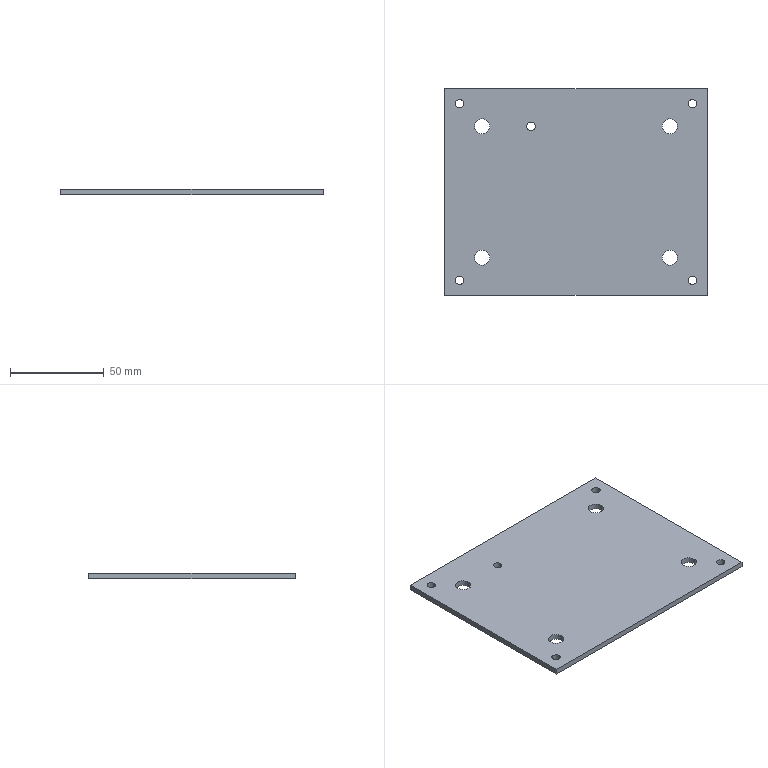Part | SolidWorks | features Extrusion 1 | 1 solid | 24 faces | box 140 x 110 x 3 mm | volume 45343 mm3 | cylinder 18 | plane 6 | commonest cylinder face diameters 4.5 x10 8.1 x8
STEP:
#1=CARTESIAN_POINT('',(-26.25,35.,-1.5));
#2=VERTEX_POINT('',#1);
#3=CARTESIAN_POINT('',(-21.75,35.,-1.5));
#4=VERTEX_POINT('',#3);
#5=CARTESIAN_POINT('',(-24.,35.,-1.5));
#6=DIRECTION('',(0.,0.,1.));
#7=DIRECTION('',(1.,0.,0.));
#8=AXIS2_PLACEMENT_3D('',#5,#6,#7);
#9=CIRCLE('',#8,2.25);
#10=EDGE_CURVE('',#2,#4,#9,.T.);
#11=ORIENTED_EDGE('',*,*,#10,.F.);
#12=CARTESIAN_POINT('',(-26.25,35.,1.5));
#13=VERTEX_POINT('',#12);
#14=CARTESIAN_POINT('',(-26.25,35.,-1.5));
#15=DIRECTION('',(0.,0.,1.));
#16=VECTOR('',#15,1000.);
#17=LINE('',#14,#16);
#18=EDGE_CURVE('',#2,#13,#17,.T.);
#19=ORIENTED_EDGE('',*,*,#18,.T.);
#20=CARTESIAN_POINT('',(-21.75,35.,1.5));
#21=VERTEX_POINT('',#20);
#22=CARTESIAN_POINT('',(-24.,35.,1.5));
#23=DIRECTION('',(0.,0.,1.));
#24=DIRECTION('',(1.,0.,0.));
#25=AXIS2_PLACEMENT_3D('',#22,#23,#24);
#26=CIRCLE('',#25,2.25);
#27=EDGE_CURVE('',#13,#21,#26,.T.);
#28=ORIENTED_EDGE('',*,*,#27,.T.);
#29=CARTESIAN_POINT('',(-21.75,35.,-1.5));
#30=DIRECTION('',(0.,0.,1.));
#31=VECTOR('',#30,1000.);
#32=LINE('',#29,#31);
#33=EDGE_CURVE('',#4,#21,#32,.T.);
#34=ORIENTED_EDGE('',*,*,#33,.F.);
#35=EDGE_LOOP('',(#11,#19,#28,#34));
#36=FACE_OUTER_BOUND('',#35,.T.);
#37=CARTESIAN_POINT('',(-24.,35.,-1.5));
#38=DIRECTION('',(0.,0.,1.));
#39=DIRECTION('',(1.,0.,0.));
#40=AXIS2_PLACEMENT_3D('',#37,#38,#39);
#41=CYLINDRICAL_SURFACE('',#40,2.25);
#42=ADVANCED_FACE('',(#36),#41,.F.);
#43=CARTESIAN_POINT('',(45.95,35.,-1.5));
#44=VERTEX_POINT('',#43);
#45=CARTESIAN_POINT('',(54.05,35.,-1.5));
#46=VERTEX_POINT('',#45);
#47=CARTESIAN_POINT('',(50.,35.,-1.5));
#48=DIRECTION('',(0.,0.,1.));
#49=DIRECTION('',(1.,0.,0.));
#50=AXIS2_PLACEMENT_3D('',#47,#48,#49);
#51=CIRCLE('',#50,4.05);
#52=EDGE_CURVE('',#44,#46,#51,.T.);
#53=ORIENTED_EDGE('',*,*,#52,.F.);
#54=CARTESIAN_POINT('',(45.95,35.,1.5));
#55=VERTEX_POINT('',#54);
#56=CARTESIAN_POINT('',(45.95,35.,-1.5));
#57=DIRECTION('',(0.,0.,1.));
#58=VECTOR('',#57,1000.);
#59=LINE('',#56,#58);
#60=EDGE_CURVE('',#44,#55,#59,.T.);
#61=ORIENTED_EDGE('',*,*,#60,.T.);
#62=CARTESIAN_POINT('',(54.05,35.,1.5));
#63=VERTEX_POINT('',#62);
#64=CARTESIAN_POINT('',(50.,35.,1.5));
#65=DIRECTION('',(0.,0.,1.));
#66=DIRECTION('',(1.,0.,0.));
#67=AXIS2_PLACEMENT_3D('',#64,#65,#66);
#68=CIRCLE('',#67,4.05);
#69=EDGE_CURVE('',#55,#63,#68,.T.);
#70=ORIENTED_EDGE('',*,*,#69,.T.);
#71=CARTESIAN_POINT('',(54.05,35.,-1.5));
#72=DIRECTION('',(0.,0.,1.));
#73=VECTOR('',#72,1000.);
#74=LINE('',#71,#73);
#75=EDGE_CURVE('',#46,#63,#74,.T.);
#76=ORIENTED_EDGE('',*,*,#75,.F.);
#77=EDGE_LOOP('',(#53,#61,#70,#76));
#78=FACE_OUTER_BOUND('',#77,.T.);
#79=CARTESIAN_POINT('',(50.,35.,-1.5));
#80=DIRECTION('',(0.,0.,1.));
#81=DIRECTION('',(1.,0.,0.));
#82=AXIS2_PLACEMENT_3D('',#79,#80,#81);
#83=CYLINDRICAL_SURFACE('',#82,4.05);
#84=ADVANCED_FACE('',(#78),#83,.F.);
#85=CARTESIAN_POINT('',(45.95,-35.,-1.5));
#86=VERTEX_POINT('',#85);
#87=CARTESIAN_POINT('',(54.05,-35.,-1.5));
#88=VERTEX_POINT('',#87);
#89=CARTESIAN_POINT('',(50.,-35.,-1.5));
#90=DIRECTION('',(0.,0.,1.));
#91=DIRECTION('',(1.,0.,0.));
#92=AXIS2_PLACEMENT_3D('',#89,#90,#91);
#93=CIRCLE('',#92,4.05);
#94=EDGE_CURVE('',#86,#88,#93,.T.);
#95=ORIENTED_EDGE('',*,*,#94,.F.);
#96=CARTESIAN_POINT('',(45.95,-35.,1.5));
#97=VERTEX_POINT('',#96);
#98=CARTESIAN_POINT('',(45.95,-35.,-1.5));
#99=DIRECTION('',(0.,0.,1.));
#100=VECTOR('',#99,1000.);
#101=LINE('',#98,#100);
#102=EDGE_CURVE('',#86,#97,#101,.T.);
#103=ORIENTED_EDGE('',*,*,#102,.T.);
#104=CARTESIAN_POINT('',(54.05,-35.,1.5));
#105=VERTEX_POINT('',#104);
#106=CARTESIAN_POINT('',(50.,-35.,1.5));
#107=DIRECTION('',(0.,0.,1.));
#108=DIRECTION('',(1.,0.,0.));
#109=AXIS2_PLACEMENT_3D('',#106,#107,#108);
#110=CIRCLE('',#109,4.05);
#111=EDGE_CURVE('',#97,#105,#110,.T.);
#112=ORIENTED_EDGE('',*,*,#111,.T.);
#113=CARTESIAN_POINT('',(54.05,-35.,-1.5));
#114=DIRECTION('',(0.,0.,1.));
#115=VECTOR('',#114,1000.);
#116=LINE('',#113,#115);
#117=EDGE_CURVE('',#88,#105,#116,.T.);
#118=ORIENTED_EDGE('',*,*,#117,.F.);
#119=EDGE_LOOP('',(#95,#103,#112,#118));
#120=FACE_OUTER_BOUND('',#119,.T.);
#121=CARTESIAN_POINT('',(50.,-35.,-1.5));
#122=DIRECTION('',(0.,0.,1.));
#123=DIRECTION('',(1.,0.,0.));
#124=AXIS2_PLACEMENT_3D('',#121,#122,#123);
#125=CYLINDRICAL_SURFACE('',#124,4.05);
#126=ADVANCED_FACE('',(#120),#125,.F.);
#127=CARTESIAN_POINT('',(-54.05,35.,-1.5));
#128=VERTEX_POINT('',#127);
#129=CARTESIAN_POINT('',(-45.95,35.,-1.5));
#130=VERTEX_POINT('',#129);
#131=CARTESIAN_POINT('',(-50.,35.,-1.5));
#132=DIRECTION('',(0.,0.,1.));
#133=DIRECTION('',(1.,0.,0.));
#134=AXIS2_PLACEMENT_3D('',#131,#132,#133);
#135=CIRCLE('',#134,4.05);
#136=EDGE_CURVE('',#128,#130,#135,.T.);
#137=ORIENTED_EDGE('',*,*,#136,.F.);
#138=CARTESIAN_POINT('',(-54.05,35.,1.5));
#139=VERTEX_POINT('',#138);
#140=CARTESIAN_POINT('',(-54.05,35.,-1.5));
#141=DIRECTION('',(0.,0.,1.));
#142=VECTOR('',#141,1000.);
#143=LINE('',#140,#142);
#144=EDGE_CURVE('',#128,#139,#143,.T.);
#145=ORIENTED_EDGE('',*,*,#144,.T.);
#146=CARTESIAN_POINT('',(-45.95,35.,1.5));
#147=VERTEX_POINT('',#146);
#148=CARTESIAN_POINT('',(-50.,35.,1.5));
#149=DIRECTION('',(0.,0.,1.));
#150=DIRECTION('',(1.,0.,0.));
#151=AXIS2_PLACEMENT_3D('',#148,#149,#150);
#152=CIRCLE('',#151,4.05);
#153=EDGE_CURVE('',#139,#147,#152,.T.);
#154=ORIENTED_EDGE('',*,*,#153,.T.);
#155=CARTESIAN_POINT('',(-45.95,35.,-1.5));
#156=DIRECTION('',(0.,0.,1.));
#157=VECTOR('',#156,1000.);
#158=LINE('',#155,#157);
#159=EDGE_CURVE('',#130,#147,#158,.T.);
#160=ORIENTED_EDGE('',*,*,#159,.F.);
#161=EDGE_LOOP('',(#137,#145,#154,#160));
#162=FACE_OUTER_BOUND('',#161,.T.);
#163=CARTESIAN_POINT('',(-50.,35.,-1.5));
#164=DIRECTION('',(0.,0.,1.));
#165=DIRECTION('',(1.,0.,0.));
#166=AXIS2_PLACEMENT_3D('',#163,#164,#165);
#167=CYLINDRICAL_SURFACE('',#166,4.05);
#168=ADVANCED_FACE('',(#162),#167,.F.);
#169=CARTESIAN_POINT('',(-54.05,-35.,-1.5));
#170=VERTEX_POINT('',#169);
#171=CARTESIAN_POINT('',(-45.95,-35.,-1.5));
#172=VERTEX_POINT('',#171);
#173=CARTESIAN_POINT('',(-50.,-35.,-1.5));
#174=DIRECTION('',(0.,0.,1.));
#175=DIRECTION('',(1.,0.,0.));
#176=AXIS2_PLACEMENT_3D('',#173,#174,#175);
#177=CIRCLE('',#176,4.05);
#178=EDGE_CURVE('',#170,#172,#177,.T.);
#179=ORIENTED_EDGE('',*,*,#178,.F.);
#180=CARTESIAN_POINT('',(-54.05,-35.,1.5));
#181=VERTEX_POINT('',#180);
#182=CARTESIAN_POINT('',(-54.05,-35.,-1.5));
#183=DIRECTION('',(0.,0.,1.));
#184=VECTOR('',#183,1000.);
#185=LINE('',#182,#184);
#186=EDGE_CURVE('',#170,#181,#185,.T.);
#187=ORIENTED_EDGE('',*,*,#186,.T.);
#188=CARTESIAN_POINT('',(-45.95,-35.,1.5));
#189=VERTEX_POINT('',#188);
#190=CARTESIAN_POINT('',(-50.,-35.,1.5));
#191=DIRECTION('',(0.,0.,1.));
#192=DIRECTION('',(1.,0.,0.));
#193=AXIS2_PLACEMENT_3D('',#190,#191,#192);
#194=CIRCLE('',#193,4.05);
#195=EDGE_CURVE('',#181,#189,#194,.T.);
#196=ORIENTED_EDGE('',*,*,#195,.T.);
#197=CARTESIAN_POINT('',(-45.95,-35.,-1.5));
#198=DIRECTION('',(0.,0.,1.));
#199=VECTOR('',#198,1000.);
#200=LINE('',#197,#199);
#201=EDGE_CURVE('',#172,#189,#200,.T.);
#202=ORIENTED_EDGE('',*,*,#201,.F.);
#203=EDGE_LOOP('',(#179,#187,#196,#202));
#204=FACE_OUTER_BOUND('',#203,.T.);
#205=CARTESIAN_POINT('',(-50.,-35.,-1.5));
#206=DIRECTION('',(0.,0.,1.));
#207=DIRECTION('',(1.,0.,0.));
#208=AXIS2_PLACEMENT_3D('',#205,#206,#207);
#209=CYLINDRICAL_SURFACE('',#208,4.05);
#210=ADVANCED_FACE('',(#204),#209,.F.);
#211=CARTESIAN_POINT('',(59.75,47.,-1.5));
#212=VERTEX_POINT('',#211);
#213=CARTESIAN_POINT('',(64.25,47.,-1.5));
#214=VERTEX_POINT('',#213);
#215=CARTESIAN_POINT('',(62.,47.,-1.5));
#216=DIRECTION('',(0.,0.,1.));
#217=DIRECTION('',(1.,0.,0.));
#218=AXIS2_PLACEMENT_3D('',#215,#216,#217);
#219=CIRCLE('',#218,2.25);
#220=EDGE_CURVE('',#212,#214,#219,.T.);
#221=ORIENTED_EDGE('',*,*,#220,.F.);
#222=CARTESIAN_POINT('',(59.75,47.,1.5));
#223=VERTEX_POINT('',#222);
#224=CARTESIAN_POINT('',(59.75,47.,-1.5));
#225=DIRECTION('',(0.,0.,1.));
#226=VECTOR('',#225,1000.);
#227=LINE('',#224,#226);
#228=EDGE_CURVE('',#212,#223,#227,.T.);
#229=ORIENTED_EDGE('',*,*,#228,.T.);
#230=CARTESIAN_POINT('',(64.25,47.,1.5));
#231=VERTEX_POINT('',#230);
#232=CARTESIAN_POINT('',(62.,47.,1.5));
#233=DIRECTION('',(0.,0.,1.));
#234=DIRECTION('',(1.,0.,0.));
#235=AXIS2_PLACEMENT_3D('',#232,#233,#234);
#236=CIRCLE('',#235,2.25);
#237=EDGE_CURVE('',#223,#231,#236,.T.);
#238=ORIENTED_EDGE('',*,*,#237,.T.);
#239=CARTESIAN_POINT('',(64.25,47.,-1.5));
#240=DIRECTION('',(0.,0.,1.));
#241=VECTOR('',#240,1000.);
#242=LINE('',#239,#241);
#243=EDGE_CURVE('',#214,#231,#242,.T.);
#244=ORIENTED_EDGE('',*,*,#243,.F.);
#245=EDGE_LOOP('',(#221,#229,#238,#244));
#246=FACE_OUTER_BOUND('',#245,.T.);
#247=CARTESIAN_POINT('',(62.,47.,-1.5));
#248=DIRECTION('',(0.,0.,1.));
#249=DIRECTION('',(1.,0.,0.));
#250=AXIS2_PLACEMENT_3D('',#247,#248,#249);
#251=CYLINDRICAL_SURFACE('',#250,2.25);
#252=ADVANCED_FACE('',(#246),#251,.F.);
#253=CARTESIAN_POINT('',(59.75,-47.,-1.5));
#254=VERTEX_POINT('',#253);
#255=CARTESIAN_POINT('',(64.25,-47.,-1.5));
#256=VERTEX_POINT('',#255);
#257=CARTESIAN_POINT('',(62.,-47.,-1.5));
#258=DIRECTION('',(0.,0.,1.));
#259=DIRECTION('',(1.,0.,0.));
#260=AXIS2_PLACEMENT_3D('',#257,#258,#259);
#261=CIRCLE('',#260,2.25);
#262=EDGE_CURVE('',#254,#256,#261,.T.);
#263=ORIENTED_EDGE('',*,*,#262,.F.);
#264=CARTESIAN_POINT('',(59.75,-47.,1.5));
#265=VERTEX_POINT('',#264);
#266=CARTESIAN_POINT('',(59.75,-47.,-1.5));
#267=DIRECTION('',(0.,0.,1.));
#268=VECTOR('',#267,1000.);
#269=LINE('',#266,#268);
#270=EDGE_CURVE('',#254,#265,#269,.T.);
#271=ORIENTED_EDGE('',*,*,#270,.T.);
#272=CARTESIAN_POINT('',(64.25,-47.,1.5));
#273=VERTEX_POINT('',#272);
#274=CARTESIAN_POINT('',(62.,-47.,1.5));
#275=DIRECTION('',(0.,0.,1.));
#276=DIRECTION('',(1.,0.,0.));
#277=AXIS2_PLACEMENT_3D('',#274,#275,#276);
#278=CIRCLE('',#277,2.25);
#279=EDGE_CURVE('',#265,#273,#278,.T.);
#280=ORIENTED_EDGE('',*,*,#279,.T.);
#281=CARTESIAN_POINT('',(64.25,-47.,-1.5));
#282=DIRECTION('',(0.,0.,1.));
#283=VECTOR('',#282,1000.);
#284=LINE('',#281,#283);
#285=EDGE_CURVE('',#256,#273,#284,.T.);
#286=ORIENTED_EDGE('',*,*,#285,.F.);
#287=EDGE_LOOP('',(#263,#271,#280,#286));
#288=FACE_OUTER_BOUND('',#287,.T.);
#289=CARTESIAN_POINT('',(62.,-47.,-1.5));
#290=DIRECTION('',(0.,0.,1.));
#291=DIRECTION('',(1.,0.,0.));
#292=AXIS2_PLACEMENT_3D('',#289,#290,#291);
#293=CYLINDRICAL_SURFACE('',#292,2.25);
#294=ADVANCED_FACE('',(#288),#293,.F.);
#295=CARTESIAN_POINT('',(-64.25,47.,-1.5));
#296=VERTEX_POINT('',#295);
#297=CARTESIAN_POINT('',(-59.75,47.,-1.5));
#298=VERTEX_POINT('',#297);
#299=CARTESIAN_POINT('',(-62.,47.,-1.5));
#300=DIRECTION('',(0.,0.,1.));
#301=DIRECTION('',(1.,0.,0.));
#302=AXIS2_PLACEMENT_3D('',#299,#300,#301);
#303=CIRCLE('',#302,2.25);
#304=EDGE_CURVE('',#296,#298,#303,.T.);
#305=ORIENTED_EDGE('',*,*,#304,.F.);
#306=CARTESIAN_POINT('',(-64.25,47.,1.5));
#307=VERTEX_POINT('',#306);
#308=CARTESIAN_POINT('',(-64.25,47.,-1.5));
#309=DIRECTION('',(0.,0.,1.));
#310=VECTOR('',#309,1000.);
#311=LINE('',#308,#310);
#312=EDGE_CURVE('',#296,#307,#311,.T.);
#313=ORIENTED_EDGE('',*,*,#312,.T.);
#314=CARTESIAN_POINT('',(-59.75,47.,1.5));
#315=VERTEX_POINT('',#314);
#316=CARTESIAN_POINT('',(-62.,47.,1.5));
#317=DIRECTION('',(0.,0.,1.));
#318=DIRECTION('',(1.,0.,0.));
#319=AXIS2_PLACEMENT_3D('',#316,#317,#318);
#320=CIRCLE('',#319,2.25);
#321=EDGE_CURVE('',#307,#315,#320,.T.);
#322=ORIENTED_EDGE('',*,*,#321,.T.);
#323=CARTESIAN_POINT('',(-59.75,47.,-1.5));
#324=DIRECTION('',(0.,0.,1.));
#325=VECTOR('',#324,1000.);
#326=LINE('',#323,#325);
#327=EDGE_CURVE('',#298,#315,#326,.T.);
#328=ORIENTED_EDGE('',*,*,#327,.F.);
#329=EDGE_LOOP('',(#305,#313,#322,#328));
#330=FACE_OUTER_BOUND('',#329,.T.);
#331=CARTESIAN_POINT('',(-62.,47.,-1.5));
#332=DIRECTION('',(0.,0.,1.));
#333=DIRECTION('',(1.,0.,0.));
#334=AXIS2_PLACEMENT_3D('',#331,#332,#333);
#335=CYLINDRICAL_SURFACE('',#334,2.25);
#336=ADVANCED_FACE('',(#330),#335,.F.);
#337=CARTESIAN_POINT('',(-64.25,-47.,-1.5));
#338=VERTEX_POINT('',#337);
#339=CARTESIAN_POINT('',(-59.75,-47.,-1.5));
#340=VERTEX_POINT('',#339);
#341=CARTESIAN_POINT('',(-62.,-47.,-1.5));
#342=DIRECTION('',(0.,0.,1.));
#343=DIRECTION('',(1.,0.,0.));
#344=AXIS2_PLACEMENT_3D('',#341,#342,#343);
#345=CIRCLE('',#344,2.25);
#346=EDGE_CURVE('',#338,#340,#345,.T.);
#347=ORIENTED_EDGE('',*,*,#346,.F.);
#348=CARTESIAN_POINT('',(-64.25,-47.,1.5));
#349=VERTEX_POINT('',#348);
#350=CARTESIAN_POINT('',(-64.25,-47.,-1.5));
#351=DIRECTION('',(0.,0.,1.));
#352=VECTOR('',#351,1000.);
#353=LINE('',#350,#352);
#354=EDGE_CURVE('',#338,#349,#353,.T.);
#355=ORIENTED_EDGE('',*,*,#354,.T.);
#356=CARTESIAN_POINT('',(-59.75,-47.,1.5));
#357=VERTEX_POINT('',#356);
#358=CARTESIAN_POINT('',(-62.,-47.,1.5));
#359=DIRECTION('',(0.,0.,1.));
#360=DIRECTION('',(1.,0.,0.));
#361=AXIS2_PLACEMENT_3D('',#358,#359,#360);
#362=CIRCLE('',#361,2.25);
#363=EDGE_CURVE('',#349,#357,#362,.T.);
#364=ORIENTED_EDGE('',*,*,#363,.T.);
#365=CARTESIAN_POINT('',(-59.75,-47.,-1.5));
#366=DIRECTION('',(0.,0.,1.));
#367=VECTOR('',#366,1000.);
#368=LINE('',#365,#367);
#369=EDGE_CURVE('',#340,#357,#368,.T.);
#370=ORIENTED_EDGE('',*,*,#369,.F.);
#371=EDGE_LOOP('',(#347,#355,#364,#370));
#372=FACE_OUTER_BOUND('',#371,.T.);
#373=CARTESIAN_POINT('',(-62.,-47.,-1.5));
#374=DIRECTION('',(0.,0.,1.));
#375=DIRECTION('',(1.,0.,0.));
#376=AXIS2_PLACEMENT_3D('',#373,#374,#375);
#377=CYLINDRICAL_SURFACE('',#376,2.25);
#378=ADVANCED_FACE('',(#372),#377,.F.);
#379=CARTESIAN_POINT('',(-70.,55.,1.5));
#380=VERTEX_POINT('',#379);
#381=CARTESIAN_POINT('',(-70.,-55.,1.5));
#382=VERTEX_POINT('',#381);
#383=CARTESIAN_POINT('',(-70.,55.,1.5));
#384=DIRECTION('',(0.,-1.,0.));
#385=VECTOR('',#384,1000.);
#386=LINE('',#383,#385);
#387=EDGE_CURVE('',#380,#382,#386,.T.);
#388=ORIENTED_EDGE('',*,*,#387,.F.);
#389=CARTESIAN_POINT('',(-70.,55.,-1.5));
#390=VERTEX_POINT('',#389);
#391=CARTESIAN_POINT('',(-70.,55.,-1.5));
#392=DIRECTION('',(0.,0.,1.));
#393=VECTOR('',#392,1000.);
#394=LINE('',#391,#393);
#395=EDGE_CURVE('',#390,#380,#394,.T.);
#396=ORIENTED_EDGE('',*,*,#395,.F.);
#397=CARTESIAN_POINT('',(-70.,-55.,-1.5));
#398=VERTEX_POINT('',#397);
#399=CARTESIAN_POINT('',(-70.,55.,-1.5));
#400=DIRECTION('',(0.,-1.,0.));
#401=VECTOR('',#400,1000.);
#402=LINE('',#399,#401);
#403=EDGE_CURVE('',#390,#398,#402,.T.);
#404=ORIENTED_EDGE('',*,*,#403,.T.);
#405=CARTESIAN_POINT('',(-70.,-55.,-1.5));
#406=DIRECTION('',(0.,0.,1.));
#407=VECTOR('',#406,1000.);
#408=LINE('',#405,#407);
#409=EDGE_CURVE('',#398,#382,#408,.T.);
#410=ORIENTED_EDGE('',*,*,#409,.T.);
#411=EDGE_LOOP('',(#388,#396,#404,#410));
#412=FACE_OUTER_BOUND('',#411,.T.);
#413=CARTESIAN_POINT('',(-70.,55.,-1.5));
#414=DIRECTION('',(-1.,0.,0.));
#415=DIRECTION('',(0.,0.,1.));
#416=AXIS2_PLACEMENT_3D('',#413,#414,#415);
#417=PLANE('',#416);
#418=ADVANCED_FACE('',(#412),#417,.T.);
#419=CARTESIAN_POINT('',(70.,55.,1.5));
#420=VERTEX_POINT('',#419);
#421=CARTESIAN_POINT('',(70.,55.,1.5));
#422=DIRECTION('',(-1.,0.,0.));
#423=VECTOR('',#422,1000.);
#424=LINE('',#421,#423);
#425=EDGE_CURVE('',#420,#380,#424,.T.);
#426=ORIENTED_EDGE('',*,*,#425,.F.);
#427=CARTESIAN_POINT('',(70.,55.,-1.5));
#428=VERTEX_POINT('',#427);
#429=CARTESIAN_POINT('',(70.,55.,-1.5));
#430=DIRECTION('',(0.,0.,1.));
#431=VECTOR('',#430,1000.);
#432=LINE('',#429,#431);
#433=EDGE_CURVE('',#428,#420,#432,.T.);
#434=ORIENTED_EDGE('',*,*,#433,.F.);
#435=CARTESIAN_POINT('',(70.,55.,-1.5));
#436=DIRECTION('',(-1.,0.,0.));
#437=VECTOR('',#436,1000.);
#438=LINE('',#435,#437);
#439=EDGE_CURVE('',#428,#390,#438,.T.);
#440=ORIENTED_EDGE('',*,*,#439,.T.);
#441=ORIENTED_EDGE('',*,*,#395,.T.);
#442=EDGE_LOOP('',(#426,#434,#440,#441));
#443=FACE_OUTER_BOUND('',#442,.T.);
#444=CARTESIAN_POINT('',(70.,55.,-1.5));
#445=DIRECTION('',(0.,1.,0.));
#446=DIRECTION('',(0.,0.,1.));
#447=AXIS2_PLACEMENT_3D('',#444,#445,#446);
#448=PLANE('',#447);
#449=ADVANCED_FACE('',(#443),#448,.T.);
#450=CARTESIAN_POINT('',(70.,-55.,1.5));
#451=VERTEX_POINT('',#450);
#452=CARTESIAN_POINT('',(70.,-55.,1.5));
#453=DIRECTION('',(0.,1.,0.));
#454=VECTOR('',#453,1000.);
#455=LINE('',#452,#454);
#456=EDGE_CURVE('',#451,#420,#455,.T.);
#457=ORIENTED_EDGE('',*,*,#456,.F.);
#458=CARTESIAN_POINT('',(70.,-55.,-1.5));
#459=VERTEX_POINT('',#458);
#460=CARTESIAN_POINT('',(70.,-55.,-1.5));
#461=DIRECTION('',(0.,0.,1.));
#462=VECTOR('',#461,1000.);
#463=LINE('',#460,#462);
#464=EDGE_CURVE('',#459,#451,#463,.T.);
#465=ORIENTED_EDGE('',*,*,#464,.F.);
#466=CARTESIAN_POINT('',(70.,-55.,-1.5));
#467=DIRECTION('',(0.,1.,0.));
#468=VECTOR('',#467,1000.);
#469=LINE('',#466,#468);
#470=EDGE_CURVE('',#459,#428,#469,.T.);
#471=ORIENTED_EDGE('',*,*,#470,.T.);
#472=ORIENTED_EDGE('',*,*,#433,.T.);
#473=EDGE_LOOP('',(#457,#465,#471,#472));
#474=FACE_OUTER_BOUND('',#473,.T.);
#475=CARTESIAN_POINT('',(70.,-55.,-1.5));
#476=DIRECTION('',(1.,0.,0.));
#477=DIRECTION('',(0.,0.,-1.));
#478=AXIS2_PLACEMENT_3D('',#475,#476,#477);
#479=PLANE('',#478);
#480=ADVANCED_FACE('',(#474),#479,.T.);
#481=CARTESIAN_POINT('',(-70.,-55.,1.5));
#482=DIRECTION('',(1.,0.,0.));
#483=VECTOR('',#482,1000.);
#484=LINE('',#481,#483);
#485=EDGE_CURVE('',#382,#451,#484,.T.);
#486=ORIENTED_EDGE('',*,*,#485,.F.);
#487=ORIENTED_EDGE('',*,*,#409,.F.);
#488=CARTESIAN_POINT('',(-70.,-55.,-1.5));
#489=DIRECTION('',(1.,0.,0.));
#490=VECTOR('',#489,1000.);
#491=LINE('',#488,#490);
#492=EDGE_CURVE('',#398,#459,#491,.T.);
#493=ORIENTED_EDGE('',*,*,#492,.T.);
#494=ORIENTED_EDGE('',*,*,#464,.T.);
#495=EDGE_LOOP('',(#486,#487,#493,#494));
#496=FACE_OUTER_BOUND('',#495,.T.);
#497=CARTESIAN_POINT('',(-70.,-55.,-1.5));
#498=DIRECTION('',(0.,-1.,0.));
#499=DIRECTION('',(0.,0.,-1.));
#500=AXIS2_PLACEMENT_3D('',#497,#498,#499);
#501=PLANE('',#500);
#502=ADVANCED_FACE('',(#496),#501,.T.);
#503=CARTESIAN_POINT('',(-24.,35.,-1.5));
#504=DIRECTION('',(0.,0.,1.));
#505=DIRECTION('',(1.,0.,0.));
#506=AXIS2_PLACEMENT_3D('',#503,#504,#505);
#507=CIRCLE('',#506,2.25);
#508=EDGE_CURVE('',#4,#2,#507,.T.);
#509=ORIENTED_EDGE('',*,*,#508,.T.);
#510=ORIENTED_EDGE('',*,*,#10,.T.);
#511=EDGE_LOOP('',(#509,#510));
#512=FACE_BOUND('',#511,.T.);
#513=CARTESIAN_POINT('',(50.,35.,-1.5));
#514=DIRECTION('',(0.,0.,1.));
#515=DIRECTION('',(1.,0.,0.));
#516=AXIS2_PLACEMENT_3D('',#513,#514,#515);
#517=CIRCLE('',#516,4.05);
#518=EDGE_CURVE('',#46,#44,#517,.T.);
#519=ORIENTED_EDGE('',*,*,#518,.T.);
#520=ORIENTED_EDGE('',*,*,#52,.T.);
#521=EDGE_LOOP('',(#519,#520));
#522=FACE_BOUND('',#521,.T.);
#523=CARTESIAN_POINT('',(50.,-35.,-1.5));
#524=DIRECTION('',(0.,0.,1.));
#525=DIRECTION('',(1.,0.,0.));
#526=AXIS2_PLACEMENT_3D('',#523,#524,#525);
#527=CIRCLE('',#526,4.05);
#528=EDGE_CURVE('',#88,#86,#527,.T.);
#529=ORIENTED_EDGE('',*,*,#528,.T.);
#530=ORIENTED_EDGE('',*,*,#94,.T.);
#531=EDGE_LOOP('',(#529,#530));
#532=FACE_BOUND('',#531,.T.);
#533=CARTESIAN_POINT('',(-50.,35.,-1.5));
#534=DIRECTION('',(0.,0.,1.));
#535=DIRECTION('',(1.,0.,0.));
#536=AXIS2_PLACEMENT_3D('',#533,#534,#535);
#537=CIRCLE('',#536,4.05);
#538=EDGE_CURVE('',#130,#128,#537,.T.);
#539=ORIENTED_EDGE('',*,*,#538,.T.);
#540=ORIENTED_EDGE('',*,*,#136,.T.);
#541=EDGE_LOOP('',(#539,#540));
#542=FACE_BOUND('',#541,.T.);
#543=CARTESIAN_POINT('',(-50.,-35.,-1.5));
#544=DIRECTION('',(0.,0.,1.));
#545=DIRECTION('',(1.,0.,0.));
#546=AXIS2_PLACEMENT_3D('',#543,#544,#545);
#547=CIRCLE('',#546,4.05);
#548=EDGE_CURVE('',#172,#170,#547,.T.);
#549=ORIENTED_EDGE('',*,*,#548,.T.);
#550=ORIENTED_EDGE('',*,*,#178,.T.);
#551=EDGE_LOOP('',(#549,#550));
#552=FACE_BOUND('',#551,.T.);
#553=CARTESIAN_POINT('',(62.,47.,-1.5));
#554=DIRECTION('',(0.,0.,1.));
#555=DIRECTION('',(1.,0.,0.));
#556=AXIS2_PLACEMENT_3D('',#553,#554,#555);
#557=CIRCLE('',#556,2.25);
#558=EDGE_CURVE('',#214,#212,#557,.T.);
#559=ORIENTED_EDGE('',*,*,#558,.T.);
#560=ORIENTED_EDGE('',*,*,#220,.T.);
#561=EDGE_LOOP('',(#559,#560));
#562=FACE_BOUND('',#561,.T.);
#563=CARTESIAN_POINT('',(62.,-47.,-1.5));
#564=DIRECTION('',(0.,0.,1.));
#565=DIRECTION('',(1.,0.,0.));
#566=AXIS2_PLACEMENT_3D('',#563,#564,#565);
#567=CIRCLE('',#566,2.25);
#568=EDGE_CURVE('',#256,#254,#567,.T.);
#569=ORIENTED_EDGE('',*,*,#568,.T.);
#570=ORIENTED_EDGE('',*,*,#262,.T.);
#571=EDGE_LOOP('',(#569,#570));
#572=FACE_BOUND('',#571,.T.);
#573=CARTESIAN_POINT('',(-62.,47.,-1.5));
#574=DIRECTION('',(0.,0.,1.));
#575=DIRECTION('',(1.,0.,0.));
#576=AXIS2_PLACEMENT_3D('',#573,#574,#575);
#577=CIRCLE('',#576,2.25);
#578=EDGE_CURVE('',#298,#296,#577,.T.);
#579=ORIENTED_EDGE('',*,*,#578,.T.);
#580=ORIENTED_EDGE('',*,*,#304,.T.);
#581=EDGE_LOOP('',(#579,#580));
#582=FACE_BOUND('',#581,.T.);
#583=CARTESIAN_POINT('',(-62.,-47.,-1.5));
#584=DIRECTION('',(0.,0.,1.));
#585=DIRECTION('',(1.,0.,0.));
#586=AXIS2_PLACEMENT_3D('',#583,#584,#585);
#587=CIRCLE('',#586,2.25);
#588=EDGE_CURVE('',#340,#338,#587,.T.);
#589=ORIENTED_EDGE('',*,*,#588,.T.);
#590=ORIENTED_EDGE('',*,*,#346,.T.);
#591=EDGE_LOOP('',(#589,#590));
#592=FACE_BOUND('',#591,.T.);
#593=ORIENTED_EDGE('',*,*,#403,.F.);
#594=ORIENTED_EDGE('',*,*,#439,.F.);
#595=ORIENTED_EDGE('',*,*,#470,.F.);
#596=ORIENTED_EDGE('',*,*,#492,.F.);
#597=EDGE_LOOP('',(#593,#594,#595,#596));
#598=FACE_OUTER_BOUND('',#597,.T.);
#599=CARTESIAN_POINT('',(0.,0.,-1.5));
#600=DIRECTION('',(0.,0.,1.));
#601=DIRECTION('',(1.,0.,0.));
#602=AXIS2_PLACEMENT_3D('',#599,#600,#601);
#603=PLANE('',#602);
#604=ADVANCED_FACE('',(#512,#522,#532,#542,#552,#562,#572,#582,#592,#598),#603,.F.);
#605=CARTESIAN_POINT('',(-24.,35.,1.5));
#606=DIRECTION('',(0.,0.,1.));
#607=DIRECTION('',(1.,0.,0.));
#608=AXIS2_PLACEMENT_3D('',#605,#606,#607);
#609=CIRCLE('',#608,2.25);
#610=EDGE_CURVE('',#21,#13,#609,.T.);
#611=ORIENTED_EDGE('',*,*,#610,.F.);
#612=ORIENTED_EDGE('',*,*,#27,.F.);
#613=EDGE_LOOP('',(#611,#612));
#614=FACE_BOUND('',#613,.T.);
#615=CARTESIAN_POINT('',(50.,35.,1.5));
#616=DIRECTION('',(0.,0.,1.));
#617=DIRECTION('',(1.,0.,0.));
#618=AXIS2_PLACEMENT_3D('',#615,#616,#617);
#619=CIRCLE('',#618,4.05);
#620=EDGE_CURVE('',#63,#55,#619,.T.);
#621=ORIENTED_EDGE('',*,*,#620,.F.);
#622=ORIENTED_EDGE('',*,*,#69,.F.);
#623=EDGE_LOOP('',(#621,#622));
#624=FACE_BOUND('',#623,.T.);
#625=CARTESIAN_POINT('',(50.,-35.,1.5));
#626=DIRECTION('',(0.,0.,1.));
#627=DIRECTION('',(1.,0.,0.));
#628=AXIS2_PLACEMENT_3D('',#625,#626,#627);
#629=CIRCLE('',#628,4.05);
#630=EDGE_CURVE('',#105,#97,#629,.T.);
#631=ORIENTED_EDGE('',*,*,#630,.F.);
#632=ORIENTED_EDGE('',*,*,#111,.F.);
#633=EDGE_LOOP('',(#631,#632));
#634=FACE_BOUND('',#633,.T.);
#635=CARTESIAN_POINT('',(-50.,35.,1.5));
#636=DIRECTION('',(0.,0.,1.));
#637=DIRECTION('',(1.,0.,0.));
#638=AXIS2_PLACEMENT_3D('',#635,#636,#637);
#639=CIRCLE('',#638,4.05);
#640=EDGE_CURVE('',#147,#139,#639,.T.);
#641=ORIENTED_EDGE('',*,*,#640,.F.);
#642=ORIENTED_EDGE('',*,*,#153,.F.);
#643=EDGE_LOOP('',(#641,#642));
#644=FACE_BOUND('',#643,.T.);
#645=CARTESIAN_POINT('',(-50.,-35.,1.5));
#646=DIRECTION('',(0.,0.,1.));
#647=DIRECTION('',(1.,0.,0.));
#648=AXIS2_PLACEMENT_3D('',#645,#646,#647);
#649=CIRCLE('',#648,4.05);
#650=EDGE_CURVE('',#189,#181,#649,.T.);
#651=ORIENTED_EDGE('',*,*,#650,.F.);
#652=ORIENTED_EDGE('',*,*,#195,.F.);
#653=EDGE_LOOP('',(#651,#652));
#654=FACE_BOUND('',#653,.T.);
#655=CARTESIAN_POINT('',(62.,47.,1.5));
#656=DIRECTION('',(0.,0.,1.));
#657=DIRECTION('',(1.,0.,0.));
#658=AXIS2_PLACEMENT_3D('',#655,#656,#657);
#659=CIRCLE('',#658,2.25);
#660=EDGE_CURVE('',#231,#223,#659,.T.);
#661=ORIENTED_EDGE('',*,*,#660,.F.);
#662=ORIENTED_EDGE('',*,*,#237,.F.);
#663=EDGE_LOOP('',(#661,#662));
#664=FACE_BOUND('',#663,.T.);
#665=CARTESIAN_POINT('',(62.,-47.,1.5));
#666=DIRECTION('',(0.,0.,1.));
#667=DIRECTION('',(1.,0.,0.));
#668=AXIS2_PLACEMENT_3D('',#665,#666,#667);
#669=CIRCLE('',#668,2.25);
#670=EDGE_CURVE('',#273,#265,#669,.T.);
#671=ORIENTED_EDGE('',*,*,#670,.F.);
#672=ORIENTED_EDGE('',*,*,#279,.F.);
#673=EDGE_LOOP('',(#671,#672));
#674=FACE_BOUND('',#673,.T.);
#675=CARTESIAN_POINT('',(-62.,47.,1.5));
#676=DIRECTION('',(0.,0.,1.));
#677=DIRECTION('',(1.,0.,0.));
#678=AXIS2_PLACEMENT_3D('',#675,#676,#677);
#679=CIRCLE('',#678,2.25);
#680=EDGE_CURVE('',#315,#307,#679,.T.);
#681=ORIENTED_EDGE('',*,*,#680,.F.);
#682=ORIENTED_EDGE('',*,*,#321,.F.);
#683=EDGE_LOOP('',(#681,#682));
#684=FACE_BOUND('',#683,.T.);
#685=CARTESIAN_POINT('',(-62.,-47.,1.5));
#686=DIRECTION('',(0.,0.,1.));
#687=DIRECTION('',(1.,0.,0.));
#688=AXIS2_PLACEMENT_3D('',#685,#686,#687);
#689=CIRCLE('',#688,2.25);
#690=EDGE_CURVE('',#357,#349,#689,.T.);
#691=ORIENTED_EDGE('',*,*,#690,.F.);
#692=ORIENTED_EDGE('',*,*,#363,.F.);
#693=EDGE_LOOP('',(#691,#692));
#694=FACE_BOUND('',#693,.T.);
#695=ORIENTED_EDGE('',*,*,#387,.T.);
#696=ORIENTED_EDGE('',*,*,#485,.T.);
#697=ORIENTED_EDGE('',*,*,#456,.T.);
#698=ORIENTED_EDGE('',*,*,#425,.T.);
#699=EDGE_LOOP('',(#695,#696,#697,#698));
#700=FACE_OUTER_BOUND('',#699,.T.);
#701=CARTESIAN_POINT('',(0.,0.,1.5));
#702=DIRECTION('',(0.,0.,1.));
#703=DIRECTION('',(1.,0.,0.));
#704=AXIS2_PLACEMENT_3D('',#701,#702,#703);
#705=PLANE('',#704);
#706=ADVANCED_FACE('',(#614,#624,#634,#644,#654,#664,#674,#684,#694,#700),#705,.T.);
#707=ORIENTED_EDGE('',*,*,#354,.F.);
#708=ORIENTED_EDGE('',*,*,#588,.F.);
#709=ORIENTED_EDGE('',*,*,#369,.T.);
#710=ORIENTED_EDGE('',*,*,#690,.T.);
#711=EDGE_LOOP('',(#707,#708,#709,#710));
#712=FACE_OUTER_BOUND('',#711,.T.);
#713=CARTESIAN_POINT('',(-62.,-47.,-1.5));
#714=DIRECTION('',(0.,0.,1.));
#715=DIRECTION('',(1.,0.,0.));
#716=AXIS2_PLACEMENT_3D('',#713,#714,#715);
#717=CYLINDRICAL_SURFACE('',#716,2.25);
#718=ADVANCED_FACE('',(#712),#717,.F.);
#719=ORIENTED_EDGE('',*,*,#312,.F.);
#720=ORIENTED_EDGE('',*,*,#578,.F.);
#721=ORIENTED_EDGE('',*,*,#327,.T.);
#722=ORIENTED_EDGE('',*,*,#680,.T.);
#723=EDGE_LOOP('',(#719,#720,#721,#722));
#724=FACE_OUTER_BOUND('',#723,.T.);
#725=CARTESIAN_POINT('',(-62.,47.,-1.5));
#726=DIRECTION('',(0.,0.,1.));
#727=DIRECTION('',(1.,0.,0.));
#728=AXIS2_PLACEMENT_3D('',#725,#726,#727);
#729=CYLINDRICAL_SURFACE('',#728,2.25);
#730=ADVANCED_FACE('',(#724),#729,.F.);
#731=ORIENTED_EDGE('',*,*,#270,.F.);
#732=ORIENTED_EDGE('',*,*,#568,.F.);
#733=ORIENTED_EDGE('',*,*,#285,.T.);
#734=ORIENTED_EDGE('',*,*,#670,.T.);
#735=EDGE_LOOP('',(#731,#732,#733,#734));
#736=FACE_OUTER_BOUND('',#735,.T.);
#737=CARTESIAN_POINT('',(62.,-47.,-1.5));
#738=DIRECTION('',(0.,0.,1.));
#739=DIRECTION('',(1.,0.,0.));
#740=AXIS2_PLACEMENT_3D('',#737,#738,#739);
#741=CYLINDRICAL_SURFACE('',#740,2.25);
#742=ADVANCED_FACE('',(#736),#741,.F.);
#743=ORIENTED_EDGE('',*,*,#228,.F.);
#744=ORIENTED_EDGE('',*,*,#558,.F.);
#745=ORIENTED_EDGE('',*,*,#243,.T.);
#746=ORIENTED_EDGE('',*,*,#660,.T.);
#747=EDGE_LOOP('',(#743,#744,#745,#746));
#748=FACE_OUTER_BOUND('',#747,.T.);
#749=CARTESIAN_POINT('',(62.,47.,-1.5));
#750=DIRECTION('',(0.,0.,1.));
#751=DIRECTION('',(1.,0.,0.));
#752=AXIS2_PLACEMENT_3D('',#749,#750,#751);
#753=CYLINDRICAL_SURFACE('',#752,2.25);
#754=ADVANCED_FACE('',(#748),#753,.F.);
#755=ORIENTED_EDGE('',*,*,#186,.F.);
#756=ORIENTED_EDGE('',*,*,#548,.F.);
#757=ORIENTED_EDGE('',*,*,#201,.T.);
#758=ORIENTED_EDGE('',*,*,#650,.T.);
#759=EDGE_LOOP('',(#755,#756,#757,#758));
#760=FACE_OUTER_BOUND('',#759,.T.);
#761=CARTESIAN_POINT('',(-50.,-35.,-1.5));
#762=DIRECTION('',(0.,0.,1.));
#763=DIRECTION('',(1.,0.,0.));
#764=AXIS2_PLACEMENT_3D('',#761,#762,#763);
#765=CYLINDRICAL_SURFACE('',#764,4.05);
#766=ADVANCED_FACE('',(#760),#765,.F.);
#767=ORIENTED_EDGE('',*,*,#144,.F.);
#768=ORIENTED_EDGE('',*,*,#538,.F.);
#769=ORIENTED_EDGE('',*,*,#159,.T.);
#770=ORIENTED_EDGE('',*,*,#640,.T.);
#771=EDGE_LOOP('',(#767,#768,#769,#770));
#772=FACE_OUTER_BOUND('',#771,.T.);
#773=CARTESIAN_POINT('',(-50.,35.,-1.5));
#774=DIRECTION('',(0.,0.,1.));
#775=DIRECTION('',(1.,0.,0.));
#776=AXIS2_PLACEMENT_3D('',#773,#774,#775);
#777=CYLINDRICAL_SURFACE('',#776,4.05);
#778=ADVANCED_FACE('',(#772),#777,.F.);
#779=ORIENTED_EDGE('',*,*,#102,.F.);
#780=ORIENTED_EDGE('',*,*,#528,.F.);
#781=ORIENTED_EDGE('',*,*,#117,.T.);
#782=ORIENTED_EDGE('',*,*,#630,.T.);
#783=EDGE_LOOP('',(#779,#780,#781,#782));
#784=FACE_OUTER_BOUND('',#783,.T.);
#785=CARTESIAN_POINT('',(50.,-35.,-1.5));
#786=DIRECTION('',(0.,0.,1.));
#787=DIRECTION('',(1.,0.,0.));
#788=AXIS2_PLACEMENT_3D('',#785,#786,#787);
#789=CYLINDRICAL_SURFACE('',#788,4.05);
#790=ADVANCED_FACE('',(#784),#789,.F.);
#791=ORIENTED_EDGE('',*,*,#60,.F.);
#792=ORIENTED_EDGE('',*,*,#518,.F.);
#793=ORIENTED_EDGE('',*,*,#75,.T.);
#794=ORIENTED_EDGE('',*,*,#620,.T.);
#795=EDGE_LOOP('',(#791,#792,#793,#794));
#796=FACE_OUTER_BOUND('',#795,.T.);
#797=CARTESIAN_POINT('',(50.,35.,-1.5));
#798=DIRECTION('',(0.,0.,1.));
#799=DIRECTION('',(1.,0.,0.));
#800=AXIS2_PLACEMENT_3D('',#797,#798,#799);
#801=CYLINDRICAL_SURFACE('',#800,4.05);
#802=ADVANCED_FACE('',(#796),#801,.F.);
#803=ORIENTED_EDGE('',*,*,#18,.F.);
#804=ORIENTED_EDGE('',*,*,#508,.F.);
#805=ORIENTED_EDGE('',*,*,#33,.T.);
#806=ORIENTED_EDGE('',*,*,#610,.T.);
#807=EDGE_LOOP('',(#803,#804,#805,#806));
#808=FACE_OUTER_BOUND('',#807,.T.);
#809=CARTESIAN_POINT('',(-24.,35.,-1.5));
#810=DIRECTION('',(0.,0.,1.));
#811=DIRECTION('',(1.,0.,0.));
#812=AXIS2_PLACEMENT_3D('',#809,#810,#811);
#813=CYLINDRICAL_SURFACE('',#812,2.25);
#814=ADVANCED_FACE('',(#808),#813,.F.);
#815=CLOSED_SHELL('',(#42,#84,#126,#168,#210,#252,#294,#336,#378,#418,#449,#480,#502,#604,#706,#718,#730,#742,#754,#766,#778,#790,#802,#814));
#816=MANIFOLD_SOLID_BREP('',#815);
#817=CARTESIAN_POINT('',(0.,0.,0.));
#818=DIRECTION('',(0.,0.,1.));
#819=DIRECTION('',(1.,0.,0.));
#820=AXIS2_PLACEMENT_3D('',#817,#818,#819);
#821=(LENGTH_UNIT()NAMED_UNIT(*)SI_UNIT(.MILLI.,.METRE.));
#822=UNCERTAINTY_MEASURE_WITH_UNIT(LENGTH_MEASURE(0.00001),#821,'','');
#823=(NAMED_UNIT(*)PLANE_ANGLE_UNIT()SI_UNIT($,.RADIAN.));
#824=(NAMED_UNIT(*)SI_UNIT($,.STERADIAN.)SOLID_ANGLE_UNIT());
#825=(GEOMETRIC_REPRESENTATION_CONTEXT(3)GLOBAL_UNCERTAINTY_ASSIGNED_CONTEXT((#822))GLOBAL_UNIT_ASSIGNED_CONTEXT((#821,#823,#824))REPRESENTATION_CONTEXT('',''));
#826=ADVANCED_BREP_SHAPE_REPRESENTATION('',(#816,#820),#825);